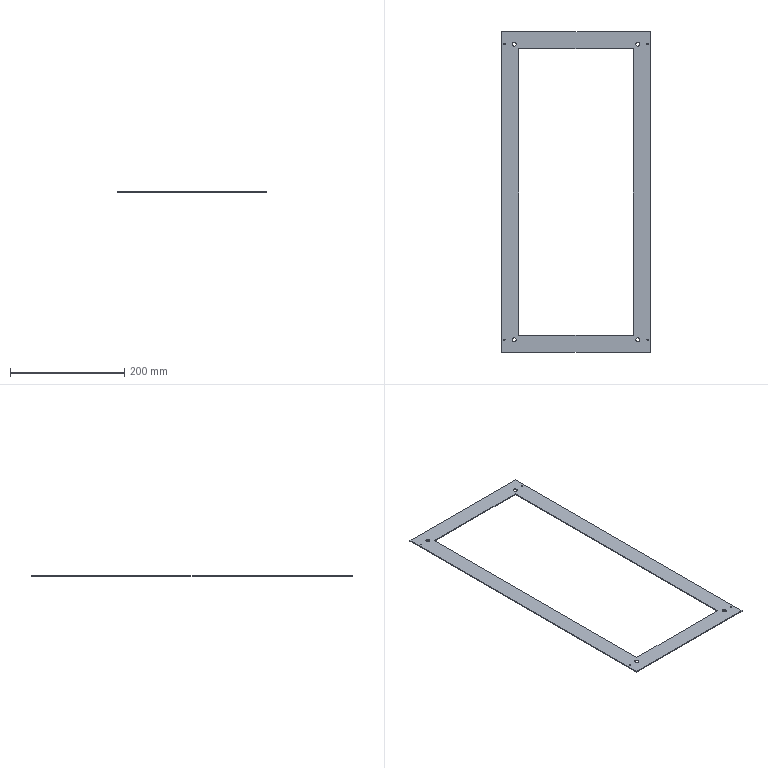Part | SolidWorks | features Cut 2, FlatPattern 1, LPattern 1, SMBaseFlange 1, SheetMetal 1 | 1 solid | 26 faces | box 260 x 560.2 x 1.5 mm | volume 68162 mm3 | cylinder 16 | plane 10 | commonest cylinder face diameters 2 x8 7.1 x8
STEP:
#1=CARTESIAN_POINT('',(234.45,538.2,-1.5));
#2=VERTEX_POINT('',#1);
#3=CARTESIAN_POINT('',(241.55,538.2,-1.5));
#4=VERTEX_POINT('',#3);
#5=CARTESIAN_POINT('',(238.,538.2,-1.5));
#6=DIRECTION('',(0.,0.,1.));
#7=DIRECTION('',(1.,0.,0.));
#8=AXIS2_PLACEMENT_3D('',#5,#6,#7);
#9=CIRCLE('',#8,3.55);
#10=EDGE_CURVE('',#2,#4,#9,.T.);
#11=ORIENTED_EDGE('',*,*,#10,.F.);
#12=CARTESIAN_POINT('',(234.45,538.2,0.));
#13=VERTEX_POINT('',#12);
#14=CARTESIAN_POINT('',(234.45,538.2,-1.5));
#15=DIRECTION('',(0.,0.,1.));
#16=VECTOR('',#15,1000.);
#17=LINE('',#14,#16);
#18=EDGE_CURVE('',#2,#13,#17,.T.);
#19=ORIENTED_EDGE('',*,*,#18,.T.);
#20=CARTESIAN_POINT('',(241.55,538.2,0.));
#21=VERTEX_POINT('',#20);
#22=CARTESIAN_POINT('',(238.,538.2,0.));
#23=DIRECTION('',(0.,0.,1.));
#24=DIRECTION('',(1.,0.,0.));
#25=AXIS2_PLACEMENT_3D('',#22,#23,#24);
#26=CIRCLE('',#25,3.55);
#27=EDGE_CURVE('',#13,#21,#26,.T.);
#28=ORIENTED_EDGE('',*,*,#27,.T.);
#29=CARTESIAN_POINT('',(241.55,538.2,-1.5));
#30=DIRECTION('',(0.,0.,1.));
#31=VECTOR('',#30,1000.);
#32=LINE('',#29,#31);
#33=EDGE_CURVE('',#4,#21,#32,.T.);
#34=ORIENTED_EDGE('',*,*,#33,.F.);
#35=EDGE_LOOP('',(#11,#19,#28,#34));
#36=FACE_OUTER_BOUND('',#35,.T.);
#37=CARTESIAN_POINT('',(238.,538.2,-1.5));
#38=DIRECTION('',(0.,0.,1.));
#39=DIRECTION('',(1.,0.,0.));
#40=AXIS2_PLACEMENT_3D('',#37,#38,#39);
#41=CYLINDRICAL_SURFACE('',#40,3.55);
#42=ADVANCED_FACE('',(#36),#41,.F.);
#43=CARTESIAN_POINT('',(18.45,538.2,-1.5));
#44=VERTEX_POINT('',#43);
#45=CARTESIAN_POINT('',(25.55,538.2,-1.5));
#46=VERTEX_POINT('',#45);
#47=CARTESIAN_POINT('',(22.,538.2,-1.5));
#48=DIRECTION('',(0.,0.,1.));
#49=DIRECTION('',(1.,0.,0.));
#50=AXIS2_PLACEMENT_3D('',#47,#48,#49);
#51=CIRCLE('',#50,3.55);
#52=EDGE_CURVE('',#44,#46,#51,.T.);
#53=ORIENTED_EDGE('',*,*,#52,.F.);
#54=CARTESIAN_POINT('',(18.45,538.2,0.));
#55=VERTEX_POINT('',#54);
#56=CARTESIAN_POINT('',(18.45,538.2,-1.5));
#57=DIRECTION('',(0.,0.,1.));
#58=VECTOR('',#57,1000.);
#59=LINE('',#56,#58);
#60=EDGE_CURVE('',#44,#55,#59,.T.);
#61=ORIENTED_EDGE('',*,*,#60,.T.);
#62=CARTESIAN_POINT('',(25.55,538.2,0.));
#63=VERTEX_POINT('',#62);
#64=CARTESIAN_POINT('',(22.,538.2,0.));
#65=DIRECTION('',(0.,0.,1.));
#66=DIRECTION('',(1.,0.,0.));
#67=AXIS2_PLACEMENT_3D('',#64,#65,#66);
#68=CIRCLE('',#67,3.55);
#69=EDGE_CURVE('',#55,#63,#68,.T.);
#70=ORIENTED_EDGE('',*,*,#69,.T.);
#71=CARTESIAN_POINT('',(25.55,538.2,-1.5));
#72=DIRECTION('',(0.,0.,1.));
#73=VECTOR('',#72,1000.);
#74=LINE('',#71,#73);
#75=EDGE_CURVE('',#46,#63,#74,.T.);
#76=ORIENTED_EDGE('',*,*,#75,.F.);
#77=EDGE_LOOP('',(#53,#61,#70,#76));
#78=FACE_OUTER_BOUND('',#77,.T.);
#79=CARTESIAN_POINT('',(22.,538.2,-1.5));
#80=DIRECTION('',(0.,0.,1.));
#81=DIRECTION('',(1.,0.,0.));
#82=AXIS2_PLACEMENT_3D('',#79,#80,#81);
#83=CYLINDRICAL_SURFACE('',#82,3.55);
#84=ADVANCED_FACE('',(#78),#83,.F.);
#85=CARTESIAN_POINT('',(18.45,22.,-1.5));
#86=VERTEX_POINT('',#85);
#87=CARTESIAN_POINT('',(25.55,22.,-1.5));
#88=VERTEX_POINT('',#87);
#89=CARTESIAN_POINT('',(22.,22.,-1.5));
#90=DIRECTION('',(0.,0.,1.));
#91=DIRECTION('',(1.,0.,0.));
#92=AXIS2_PLACEMENT_3D('',#89,#90,#91);
#93=CIRCLE('',#92,3.55);
#94=EDGE_CURVE('',#86,#88,#93,.T.);
#95=ORIENTED_EDGE('',*,*,#94,.F.);
#96=CARTESIAN_POINT('',(18.45,22.,0.));
#97=VERTEX_POINT('',#96);
#98=CARTESIAN_POINT('',(18.45,22.,-1.5));
#99=DIRECTION('',(0.,0.,1.));
#100=VECTOR('',#99,1000.);
#101=LINE('',#98,#100);
#102=EDGE_CURVE('',#86,#97,#101,.T.);
#103=ORIENTED_EDGE('',*,*,#102,.T.);
#104=CARTESIAN_POINT('',(25.55,22.,0.));
#105=VERTEX_POINT('',#104);
#106=CARTESIAN_POINT('',(22.,22.,0.));
#107=DIRECTION('',(0.,0.,1.));
#108=DIRECTION('',(1.,0.,0.));
#109=AXIS2_PLACEMENT_3D('',#106,#107,#108);
#110=CIRCLE('',#109,3.55);
#111=EDGE_CURVE('',#97,#105,#110,.T.);
#112=ORIENTED_EDGE('',*,*,#111,.T.);
#113=CARTESIAN_POINT('',(25.55,22.,-1.5));
#114=DIRECTION('',(0.,0.,1.));
#115=VECTOR('',#114,1000.);
#116=LINE('',#113,#115);
#117=EDGE_CURVE('',#88,#105,#116,.T.);
#118=ORIENTED_EDGE('',*,*,#117,.F.);
#119=EDGE_LOOP('',(#95,#103,#112,#118));
#120=FACE_OUTER_BOUND('',#119,.T.);
#121=CARTESIAN_POINT('',(22.,22.,-1.5));
#122=DIRECTION('',(0.,0.,1.));
#123=DIRECTION('',(1.,0.,0.));
#124=AXIS2_PLACEMENT_3D('',#121,#122,#123);
#125=CYLINDRICAL_SURFACE('',#124,3.55);
#126=ADVANCED_FACE('',(#120),#125,.F.);
#127=CARTESIAN_POINT('',(234.45,22.,-1.5));
#128=VERTEX_POINT('',#127);
#129=CARTESIAN_POINT('',(241.55,22.,-1.5));
#130=VERTEX_POINT('',#129);
#131=CARTESIAN_POINT('',(238.,22.,-1.5));
#132=DIRECTION('',(0.,0.,1.));
#133=DIRECTION('',(1.,0.,0.));
#134=AXIS2_PLACEMENT_3D('',#131,#132,#133);
#135=CIRCLE('',#134,3.55);
#136=EDGE_CURVE('',#128,#130,#135,.T.);
#137=ORIENTED_EDGE('',*,*,#136,.F.);
#138=CARTESIAN_POINT('',(234.45,22.,0.));
#139=VERTEX_POINT('',#138);
#140=CARTESIAN_POINT('',(234.45,22.,-1.5));
#141=DIRECTION('',(0.,0.,1.));
#142=VECTOR('',#141,1000.);
#143=LINE('',#140,#142);
#144=EDGE_CURVE('',#128,#139,#143,.T.);
#145=ORIENTED_EDGE('',*,*,#144,.T.);
#146=CARTESIAN_POINT('',(241.55,22.,0.));
#147=VERTEX_POINT('',#146);
#148=CARTESIAN_POINT('',(238.,22.,0.));
#149=DIRECTION('',(0.,0.,1.));
#150=DIRECTION('',(1.,0.,0.));
#151=AXIS2_PLACEMENT_3D('',#148,#149,#150);
#152=CIRCLE('',#151,3.55);
#153=EDGE_CURVE('',#139,#147,#152,.T.);
#154=ORIENTED_EDGE('',*,*,#153,.T.);
#155=CARTESIAN_POINT('',(241.55,22.,-1.5));
#156=DIRECTION('',(0.,0.,1.));
#157=VECTOR('',#156,1000.);
#158=LINE('',#155,#157);
#159=EDGE_CURVE('',#130,#147,#158,.T.);
#160=ORIENTED_EDGE('',*,*,#159,.F.);
#161=EDGE_LOOP('',(#137,#145,#154,#160));
#162=FACE_OUTER_BOUND('',#161,.T.);
#163=CARTESIAN_POINT('',(238.,22.,-1.5));
#164=DIRECTION('',(0.,0.,1.));
#165=DIRECTION('',(1.,0.,0.));
#166=AXIS2_PLACEMENT_3D('',#163,#164,#165);
#167=CYLINDRICAL_SURFACE('',#166,3.55);
#168=ADVANCED_FACE('',(#162),#167,.F.);
#169=CARTESIAN_POINT('',(4.,22.,-1.5));
#170=VERTEX_POINT('',#169);
#171=CARTESIAN_POINT('',(6.,22.,-1.5));
#172=VERTEX_POINT('',#171);
#173=CARTESIAN_POINT('',(5.,22.,-1.5));
#174=DIRECTION('',(0.,0.,1.));
#175=DIRECTION('',(1.,0.,0.));
#176=AXIS2_PLACEMENT_3D('',#173,#174,#175);
#177=CIRCLE('',#176,1.);
#178=EDGE_CURVE('',#170,#172,#177,.T.);
#179=ORIENTED_EDGE('',*,*,#178,.F.);
#180=CARTESIAN_POINT('',(4.,22.,0.));
#181=VERTEX_POINT('',#180);
#182=CARTESIAN_POINT('',(4.,22.,-1.5));
#183=DIRECTION('',(0.,0.,1.));
#184=VECTOR('',#183,1000.);
#185=LINE('',#182,#184);
#186=EDGE_CURVE('',#170,#181,#185,.T.);
#187=ORIENTED_EDGE('',*,*,#186,.T.);
#188=CARTESIAN_POINT('',(6.,22.,0.));
#189=VERTEX_POINT('',#188);
#190=CARTESIAN_POINT('',(5.,22.,0.));
#191=DIRECTION('',(0.,0.,1.));
#192=DIRECTION('',(1.,0.,0.));
#193=AXIS2_PLACEMENT_3D('',#190,#191,#192);
#194=CIRCLE('',#193,1.);
#195=EDGE_CURVE('',#181,#189,#194,.T.);
#196=ORIENTED_EDGE('',*,*,#195,.T.);
#197=CARTESIAN_POINT('',(6.,22.,-1.5));
#198=DIRECTION('',(0.,0.,1.));
#199=VECTOR('',#198,1000.);
#200=LINE('',#197,#199);
#201=EDGE_CURVE('',#172,#189,#200,.T.);
#202=ORIENTED_EDGE('',*,*,#201,.F.);
#203=EDGE_LOOP('',(#179,#187,#196,#202));
#204=FACE_OUTER_BOUND('',#203,.T.);
#205=CARTESIAN_POINT('',(5.,22.,-1.5));
#206=DIRECTION('',(0.,0.,1.));
#207=DIRECTION('',(1.,0.,0.));
#208=AXIS2_PLACEMENT_3D('',#205,#206,#207);
#209=CYLINDRICAL_SURFACE('',#208,1.);
#210=ADVANCED_FACE('',(#204),#209,.F.);
#211=CARTESIAN_POINT('',(254.,22.,-1.5));
#212=VERTEX_POINT('',#211);
#213=CARTESIAN_POINT('',(256.,22.,-1.5));
#214=VERTEX_POINT('',#213);
#215=CARTESIAN_POINT('',(255.,22.,-1.5));
#216=DIRECTION('',(0.,0.,1.));
#217=DIRECTION('',(1.,0.,0.));
#218=AXIS2_PLACEMENT_3D('',#215,#216,#217);
#219=CIRCLE('',#218,1.);
#220=EDGE_CURVE('',#212,#214,#219,.T.);
#221=ORIENTED_EDGE('',*,*,#220,.F.);
#222=CARTESIAN_POINT('',(254.,22.,0.));
#223=VERTEX_POINT('',#222);
#224=CARTESIAN_POINT('',(254.,22.,-1.5));
#225=DIRECTION('',(0.,0.,1.));
#226=VECTOR('',#225,1000.);
#227=LINE('',#224,#226);
#228=EDGE_CURVE('',#212,#223,#227,.T.);
#229=ORIENTED_EDGE('',*,*,#228,.T.);
#230=CARTESIAN_POINT('',(256.,22.,0.));
#231=VERTEX_POINT('',#230);
#232=CARTESIAN_POINT('',(255.,22.,0.));
#233=DIRECTION('',(0.,0.,1.));
#234=DIRECTION('',(1.,0.,0.));
#235=AXIS2_PLACEMENT_3D('',#232,#233,#234);
#236=CIRCLE('',#235,1.);
#237=EDGE_CURVE('',#223,#231,#236,.T.);
#238=ORIENTED_EDGE('',*,*,#237,.T.);
#239=CARTESIAN_POINT('',(256.,22.,-1.5));
#240=DIRECTION('',(0.,0.,1.));
#241=VECTOR('',#240,1000.);
#242=LINE('',#239,#241);
#243=EDGE_CURVE('',#214,#231,#242,.T.);
#244=ORIENTED_EDGE('',*,*,#243,.F.);
#245=EDGE_LOOP('',(#221,#229,#238,#244));
#246=FACE_OUTER_BOUND('',#245,.T.);
#247=CARTESIAN_POINT('',(255.,22.,-1.5));
#248=DIRECTION('',(0.,0.,1.));
#249=DIRECTION('',(1.,0.,0.));
#250=AXIS2_PLACEMENT_3D('',#247,#248,#249);
#251=CYLINDRICAL_SURFACE('',#250,1.);
#252=ADVANCED_FACE('',(#246),#251,.F.);
#253=CARTESIAN_POINT('',(254.,538.6,-1.5));
#254=VERTEX_POINT('',#253);
#255=CARTESIAN_POINT('',(256.,538.6,-1.5));
#256=VERTEX_POINT('',#255);
#257=CARTESIAN_POINT('',(255.,538.6,-1.5));
#258=DIRECTION('',(0.,0.,1.));
#259=DIRECTION('',(1.,0.,0.));
#260=AXIS2_PLACEMENT_3D('',#257,#258,#259);
#261=CIRCLE('',#260,1.);
#262=EDGE_CURVE('',#254,#256,#261,.T.);
#263=ORIENTED_EDGE('',*,*,#262,.F.);
#264=CARTESIAN_POINT('',(254.,538.6,0.));
#265=VERTEX_POINT('',#264);
#266=CARTESIAN_POINT('',(254.,538.6,-1.5));
#267=DIRECTION('',(0.,0.,1.));
#268=VECTOR('',#267,1000.);
#269=LINE('',#266,#268);
#270=EDGE_CURVE('',#254,#265,#269,.T.);
#271=ORIENTED_EDGE('',*,*,#270,.T.);
#272=CARTESIAN_POINT('',(256.,538.6,0.));
#273=VERTEX_POINT('',#272);
#274=CARTESIAN_POINT('',(255.,538.6,0.));
#275=DIRECTION('',(0.,0.,1.));
#276=DIRECTION('',(1.,0.,0.));
#277=AXIS2_PLACEMENT_3D('',#274,#275,#276);
#278=CIRCLE('',#277,1.);
#279=EDGE_CURVE('',#265,#273,#278,.T.);
#280=ORIENTED_EDGE('',*,*,#279,.T.);
#281=CARTESIAN_POINT('',(256.,538.6,-1.5));
#282=DIRECTION('',(0.,0.,1.));
#283=VECTOR('',#282,1000.);
#284=LINE('',#281,#283);
#285=EDGE_CURVE('',#256,#273,#284,.T.);
#286=ORIENTED_EDGE('',*,*,#285,.F.);
#287=EDGE_LOOP('',(#263,#271,#280,#286));
#288=FACE_OUTER_BOUND('',#287,.T.);
#289=CARTESIAN_POINT('',(255.,538.6,-1.5));
#290=DIRECTION('',(0.,0.,1.));
#291=DIRECTION('',(1.,0.,0.));
#292=AXIS2_PLACEMENT_3D('',#289,#290,#291);
#293=CYLINDRICAL_SURFACE('',#292,1.);
#294=ADVANCED_FACE('',(#288),#293,.F.);
#295=CARTESIAN_POINT('',(4.,538.6,-1.5));
#296=VERTEX_POINT('',#295);
#297=CARTESIAN_POINT('',(6.,538.6,-1.5));
#298=VERTEX_POINT('',#297);
#299=CARTESIAN_POINT('',(5.,538.6,-1.5));
#300=DIRECTION('',(0.,0.,1.));
#301=DIRECTION('',(1.,0.,0.));
#302=AXIS2_PLACEMENT_3D('',#299,#300,#301);
#303=CIRCLE('',#302,1.);
#304=EDGE_CURVE('',#296,#298,#303,.T.);
#305=ORIENTED_EDGE('',*,*,#304,.F.);
#306=CARTESIAN_POINT('',(4.,538.6,0.));
#307=VERTEX_POINT('',#306);
#308=CARTESIAN_POINT('',(4.,538.6,-1.5));
#309=DIRECTION('',(0.,0.,1.));
#310=VECTOR('',#309,1000.);
#311=LINE('',#308,#310);
#312=EDGE_CURVE('',#296,#307,#311,.T.);
#313=ORIENTED_EDGE('',*,*,#312,.T.);
#314=CARTESIAN_POINT('',(6.,538.6,0.));
#315=VERTEX_POINT('',#314);
#316=CARTESIAN_POINT('',(5.,538.6,0.));
#317=DIRECTION('',(0.,0.,1.));
#318=DIRECTION('',(1.,0.,0.));
#319=AXIS2_PLACEMENT_3D('',#316,#317,#318);
#320=CIRCLE('',#319,1.);
#321=EDGE_CURVE('',#307,#315,#320,.T.);
#322=ORIENTED_EDGE('',*,*,#321,.T.);
#323=CARTESIAN_POINT('',(6.,538.6,-1.5));
#324=DIRECTION('',(0.,0.,1.));
#325=VECTOR('',#324,1000.);
#326=LINE('',#323,#325);
#327=EDGE_CURVE('',#298,#315,#326,.T.);
#328=ORIENTED_EDGE('',*,*,#327,.F.);
#329=EDGE_LOOP('',(#305,#313,#322,#328));
#330=FACE_OUTER_BOUND('',#329,.T.);
#331=CARTESIAN_POINT('',(5.,538.6,-1.5));
#332=DIRECTION('',(0.,0.,1.));
#333=DIRECTION('',(1.,0.,0.));
#334=AXIS2_PLACEMENT_3D('',#331,#332,#333);
#335=CYLINDRICAL_SURFACE('',#334,1.);
#336=ADVANCED_FACE('',(#330),#335,.F.);
#337=ORIENTED_EDGE('',*,*,#312,.F.);
#338=CARTESIAN_POINT('',(5.,538.6,-1.5));
#339=DIRECTION('',(0.,0.,1.));
#340=DIRECTION('',(1.,0.,0.));
#341=AXIS2_PLACEMENT_3D('',#338,#339,#340);
#342=CIRCLE('',#341,1.);
#343=EDGE_CURVE('',#298,#296,#342,.T.);
#344=ORIENTED_EDGE('',*,*,#343,.F.);
#345=ORIENTED_EDGE('',*,*,#327,.T.);
#346=CARTESIAN_POINT('',(5.,538.6,0.));
#347=DIRECTION('',(0.,0.,1.));
#348=DIRECTION('',(1.,0.,0.));
#349=AXIS2_PLACEMENT_3D('',#346,#347,#348);
#350=CIRCLE('',#349,1.);
#351=EDGE_CURVE('',#315,#307,#350,.T.);
#352=ORIENTED_EDGE('',*,*,#351,.T.);
#353=EDGE_LOOP('',(#337,#344,#345,#352));
#354=FACE_OUTER_BOUND('',#353,.T.);
#355=CARTESIAN_POINT('',(5.,538.6,-1.5));
#356=DIRECTION('',(0.,0.,1.));
#357=DIRECTION('',(1.,0.,0.));
#358=AXIS2_PLACEMENT_3D('',#355,#356,#357);
#359=CYLINDRICAL_SURFACE('',#358,1.);
#360=ADVANCED_FACE('',(#354),#359,.F.);
#361=ORIENTED_EDGE('',*,*,#270,.F.);
#362=CARTESIAN_POINT('',(255.,538.6,-1.5));
#363=DIRECTION('',(0.,0.,1.));
#364=DIRECTION('',(1.,0.,0.));
#365=AXIS2_PLACEMENT_3D('',#362,#363,#364);
#366=CIRCLE('',#365,1.);
#367=EDGE_CURVE('',#256,#254,#366,.T.);
#368=ORIENTED_EDGE('',*,*,#367,.F.);
#369=ORIENTED_EDGE('',*,*,#285,.T.);
#370=CARTESIAN_POINT('',(255.,538.6,0.));
#371=DIRECTION('',(0.,0.,1.));
#372=DIRECTION('',(1.,0.,0.));
#373=AXIS2_PLACEMENT_3D('',#370,#371,#372);
#374=CIRCLE('',#373,1.);
#375=EDGE_CURVE('',#273,#265,#374,.T.);
#376=ORIENTED_EDGE('',*,*,#375,.T.);
#377=EDGE_LOOP('',(#361,#368,#369,#376));
#378=FACE_OUTER_BOUND('',#377,.T.);
#379=CARTESIAN_POINT('',(255.,538.6,-1.5));
#380=DIRECTION('',(0.,0.,1.));
#381=DIRECTION('',(1.,0.,0.));
#382=AXIS2_PLACEMENT_3D('',#379,#380,#381);
#383=CYLINDRICAL_SURFACE('',#382,1.);
#384=ADVANCED_FACE('',(#378),#383,.F.);
#385=CARTESIAN_POINT('',(0.,560.2,0.));
#386=VERTEX_POINT('',#385);
#387=CARTESIAN_POINT('',(0.,0.,0.));
#388=VERTEX_POINT('',#387);
#389=CARTESIAN_POINT('',(0.,0.,0.));
#390=DIRECTION('',(0.,-1.,0.));
#391=VECTOR('',#390,1000.);
#392=LINE('',#389,#391);
#393=EDGE_CURVE('',#386,#388,#392,.T.);
#394=ORIENTED_EDGE('',*,*,#393,.F.);
#395=CARTESIAN_POINT('',(0.,560.2,-1.5));
#396=VERTEX_POINT('',#395);
#397=CARTESIAN_POINT('',(0.,560.2,-1.5));
#398=DIRECTION('',(0.,0.,1.));
#399=VECTOR('',#398,1000.);
#400=LINE('',#397,#399);
#401=EDGE_CURVE('',#396,#386,#400,.T.);
#402=ORIENTED_EDGE('',*,*,#401,.F.);
#403=CARTESIAN_POINT('',(0.,0.,-1.5));
#404=VERTEX_POINT('',#403);
#405=CARTESIAN_POINT('',(0.,0.,-1.5));
#406=DIRECTION('',(0.,-1.,0.));
#407=VECTOR('',#406,1000.);
#408=LINE('',#405,#407);
#409=EDGE_CURVE('',#396,#404,#408,.T.);
#410=ORIENTED_EDGE('',*,*,#409,.T.);
#411=CARTESIAN_POINT('',(0.,0.,-1.5));
#412=DIRECTION('',(0.,0.,1.));
#413=VECTOR('',#412,1000.);
#414=LINE('',#411,#413);
#415=EDGE_CURVE('',#404,#388,#414,.T.);
#416=ORIENTED_EDGE('',*,*,#415,.T.);
#417=EDGE_LOOP('',(#394,#402,#410,#416));
#418=FACE_OUTER_BOUND('',#417,.T.);
#419=CARTESIAN_POINT('',(0.,0.,-1.5));
#420=DIRECTION('',(-1.,0.,0.));
#421=DIRECTION('',(0.,-1.,0.));
#422=AXIS2_PLACEMENT_3D('',#419,#420,#421);
#423=PLANE('',#422);
#424=ADVANCED_FACE('',(#418),#423,.T.);
#425=CARTESIAN_POINT('',(260.,560.2,0.));
#426=VERTEX_POINT('',#425);
#427=CARTESIAN_POINT('',(0.,560.2,0.));
#428=DIRECTION('',(-1.,0.,0.));
#429=VECTOR('',#428,1000.);
#430=LINE('',#427,#429);
#431=EDGE_CURVE('',#426,#386,#430,.T.);
#432=ORIENTED_EDGE('',*,*,#431,.F.);
#433=CARTESIAN_POINT('',(260.,560.2,-1.5));
#434=VERTEX_POINT('',#433);
#435=CARTESIAN_POINT('',(260.,560.2,-1.5));
#436=DIRECTION('',(0.,0.,1.));
#437=VECTOR('',#436,1000.);
#438=LINE('',#435,#437);
#439=EDGE_CURVE('',#434,#426,#438,.T.);
#440=ORIENTED_EDGE('',*,*,#439,.F.);
#441=CARTESIAN_POINT('',(0.,560.2,-1.5));
#442=DIRECTION('',(-1.,0.,0.));
#443=VECTOR('',#442,1000.);
#444=LINE('',#441,#443);
#445=EDGE_CURVE('',#434,#396,#444,.T.);
#446=ORIENTED_EDGE('',*,*,#445,.T.);
#447=ORIENTED_EDGE('',*,*,#401,.T.);
#448=EDGE_LOOP('',(#432,#440,#446,#447));
#449=FACE_OUTER_BOUND('',#448,.T.);
#450=CARTESIAN_POINT('',(0.,560.2,-1.5));
#451=DIRECTION('',(0.,1.,0.));
#452=DIRECTION('',(0.,0.,1.));
#453=AXIS2_PLACEMENT_3D('',#450,#451,#452);
#454=PLANE('',#453);
#455=ADVANCED_FACE('',(#449),#454,.T.);
#456=CARTESIAN_POINT('',(260.,0.,0.));
#457=VERTEX_POINT('',#456);
#458=CARTESIAN_POINT('',(260.,0.,0.));
#459=DIRECTION('',(0.,1.,0.));
#460=VECTOR('',#459,1000.);
#461=LINE('',#458,#460);
#462=EDGE_CURVE('',#457,#426,#461,.T.);
#463=ORIENTED_EDGE('',*,*,#462,.F.);
#464=CARTESIAN_POINT('',(260.,0.,-1.5));
#465=VERTEX_POINT('',#464);
#466=CARTESIAN_POINT('',(260.,0.,-1.5));
#467=DIRECTION('',(0.,0.,1.));
#468=VECTOR('',#467,1000.);
#469=LINE('',#466,#468);
#470=EDGE_CURVE('',#465,#457,#469,.T.);
#471=ORIENTED_EDGE('',*,*,#470,.F.);
#472=CARTESIAN_POINT('',(260.,0.,-1.5));
#473=DIRECTION('',(0.,1.,0.));
#474=VECTOR('',#473,1000.);
#475=LINE('',#472,#474);
#476=EDGE_CURVE('',#465,#434,#475,.T.);
#477=ORIENTED_EDGE('',*,*,#476,.T.);
#478=ORIENTED_EDGE('',*,*,#439,.T.);
#479=EDGE_LOOP('',(#463,#471,#477,#478));
#480=FACE_OUTER_BOUND('',#479,.T.);
#481=CARTESIAN_POINT('',(260.,0.,-1.5));
#482=DIRECTION('',(1.,0.,0.));
#483=DIRECTION('',(0.,1.,0.));
#484=AXIS2_PLACEMENT_3D('',#481,#482,#483);
#485=PLANE('',#484);
#486=ADVANCED_FACE('',(#480),#485,.T.);
#487=CARTESIAN_POINT('',(0.,0.,0.));
#488=DIRECTION('',(1.,0.,0.));
#489=VECTOR('',#488,1000.);
#490=LINE('',#487,#489);
#491=EDGE_CURVE('',#388,#457,#490,.T.);
#492=ORIENTED_EDGE('',*,*,#491,.F.);
#493=ORIENTED_EDGE('',*,*,#415,.F.);
#494=CARTESIAN_POINT('',(0.,0.,-1.5));
#495=DIRECTION('',(1.,0.,0.));
#496=VECTOR('',#495,1000.);
#497=LINE('',#494,#496);
#498=EDGE_CURVE('',#404,#465,#497,.T.);
#499=ORIENTED_EDGE('',*,*,#498,.T.);
#500=ORIENTED_EDGE('',*,*,#470,.T.);
#501=EDGE_LOOP('',(#492,#493,#499,#500));
#502=FACE_OUTER_BOUND('',#501,.T.);
#503=CARTESIAN_POINT('',(0.,0.,-1.5));
#504=DIRECTION('',(0.,-1.,0.));
#505=DIRECTION('',(0.,0.,-1.));
#506=AXIS2_PLACEMENT_3D('',#503,#504,#505);
#507=PLANE('',#506);
#508=ADVANCED_FACE('',(#502),#507,.T.);
#509=CARTESIAN_POINT('',(238.,538.2,-1.5));
#510=DIRECTION('',(0.,0.,1.));
#511=DIRECTION('',(1.,0.,0.));
#512=AXIS2_PLACEMENT_3D('',#509,#510,#511);
#513=CIRCLE('',#512,3.55);
#514=EDGE_CURVE('',#4,#2,#513,.T.);
#515=ORIENTED_EDGE('',*,*,#514,.T.);
#516=ORIENTED_EDGE('',*,*,#10,.T.);
#517=EDGE_LOOP('',(#515,#516));
#518=FACE_BOUND('',#517,.T.);
#519=CARTESIAN_POINT('',(22.,538.2,-1.5));
#520=DIRECTION('',(0.,0.,1.));
#521=DIRECTION('',(1.,0.,0.));
#522=AXIS2_PLACEMENT_3D('',#519,#520,#521);
#523=CIRCLE('',#522,3.55);
#524=EDGE_CURVE('',#46,#44,#523,.T.);
#525=ORIENTED_EDGE('',*,*,#524,.T.);
#526=ORIENTED_EDGE('',*,*,#52,.T.);
#527=EDGE_LOOP('',(#525,#526));
#528=FACE_BOUND('',#527,.T.);
#529=CARTESIAN_POINT('',(22.,22.,-1.5));
#530=DIRECTION('',(0.,0.,1.));
#531=DIRECTION('',(1.,0.,0.));
#532=AXIS2_PLACEMENT_3D('',#529,#530,#531);
#533=CIRCLE('',#532,3.55);
#534=EDGE_CURVE('',#88,#86,#533,.T.);
#535=ORIENTED_EDGE('',*,*,#534,.T.);
#536=ORIENTED_EDGE('',*,*,#94,.T.);
#537=EDGE_LOOP('',(#535,#536));
#538=FACE_BOUND('',#537,.T.);
#539=CARTESIAN_POINT('',(238.,22.,-1.5));
#540=DIRECTION('',(0.,0.,1.));
#541=DIRECTION('',(1.,0.,0.));
#542=AXIS2_PLACEMENT_3D('',#539,#540,#541);
#543=CIRCLE('',#542,3.55);
#544=EDGE_CURVE('',#130,#128,#543,.T.);
#545=ORIENTED_EDGE('',*,*,#544,.T.);
#546=ORIENTED_EDGE('',*,*,#136,.T.);
#547=EDGE_LOOP('',(#545,#546));
#548=FACE_BOUND('',#547,.T.);
#549=CARTESIAN_POINT('',(5.,22.,-1.5));
#550=DIRECTION('',(0.,0.,1.));
#551=DIRECTION('',(1.,0.,0.));
#552=AXIS2_PLACEMENT_3D('',#549,#550,#551);
#553=CIRCLE('',#552,1.);
#554=EDGE_CURVE('',#172,#170,#553,.T.);
#555=ORIENTED_EDGE('',*,*,#554,.T.);
#556=ORIENTED_EDGE('',*,*,#178,.T.);
#557=EDGE_LOOP('',(#555,#556));
#558=FACE_BOUND('',#557,.T.);
#559=CARTESIAN_POINT('',(255.,22.,-1.5));
#560=DIRECTION('',(0.,0.,1.));
#561=DIRECTION('',(1.,0.,0.));
#562=AXIS2_PLACEMENT_3D('',#559,#560,#561);
#563=CIRCLE('',#562,1.);
#564=EDGE_CURVE('',#214,#212,#563,.T.);
#565=ORIENTED_EDGE('',*,*,#564,.T.);
#566=ORIENTED_EDGE('',*,*,#220,.T.);
#567=EDGE_LOOP('',(#565,#566));
#568=FACE_BOUND('',#567,.T.);
#569=CARTESIAN_POINT('',(30.,530.2,-1.5));
#570=VERTEX_POINT('',#569);
#571=CARTESIAN_POINT('',(30.,30.,-1.5));
#572=VERTEX_POINT('',#571);
#573=CARTESIAN_POINT('',(30.,30.,-1.5));
#574=DIRECTION('',(0.,-1.,0.));
#575=VECTOR('',#574,1000.);
#576=LINE('',#573,#575);
#577=EDGE_CURVE('',#570,#572,#576,.T.);
#578=ORIENTED_EDGE('',*,*,#577,.T.);
#579=CARTESIAN_POINT('',(230.,30.,-1.5));
#580=VERTEX_POINT('',#579);
#581=CARTESIAN_POINT('',(30.,30.,-1.5));
#582=DIRECTION('',(1.,0.,0.));
#583=VECTOR('',#582,1000.);
#584=LINE('',#581,#583);
#585=EDGE_CURVE('',#572,#580,#584,.T.);
#586=ORIENTED_EDGE('',*,*,#585,.T.);
#587=CARTESIAN_POINT('',(230.,530.2,-1.5));
#588=VERTEX_POINT('',#587);
#589=CARTESIAN_POINT('',(230.,30.,-1.5));
#590=DIRECTION('',(0.,1.,0.));
#591=VECTOR('',#590,1000.);
#592=LINE('',#589,#591);
#593=EDGE_CURVE('',#580,#588,#592,.T.);
#594=ORIENTED_EDGE('',*,*,#593,.T.);
#595=CARTESIAN_POINT('',(30.,530.2,-1.5));
#596=DIRECTION('',(-1.,0.,0.));
#597=VECTOR('',#596,1000.);
#598=LINE('',#595,#597);
#599=EDGE_CURVE('',#588,#570,#598,.T.);
#600=ORIENTED_EDGE('',*,*,#599,.T.);
#601=EDGE_LOOP('',(#578,#586,#594,#600));
#602=FACE_BOUND('',#601,.T.);
#603=ORIENTED_EDGE('',*,*,#409,.F.);
#604=ORIENTED_EDGE('',*,*,#445,.F.);
#605=ORIENTED_EDGE('',*,*,#476,.F.);
#606=ORIENTED_EDGE('',*,*,#498,.F.);
#607=EDGE_LOOP('',(#603,#604,#605,#606));
#608=FACE_OUTER_BOUND('',#607,.T.);
#609=ORIENTED_EDGE('',*,*,#367,.T.);
#610=ORIENTED_EDGE('',*,*,#262,.T.);
#611=EDGE_LOOP('',(#609,#610));
#612=FACE_BOUND('',#611,.T.);
#613=ORIENTED_EDGE('',*,*,#343,.T.);
#614=ORIENTED_EDGE('',*,*,#304,.T.);
#615=EDGE_LOOP('',(#613,#614));
#616=FACE_BOUND('',#615,.T.);
#617=CARTESIAN_POINT('',(0.,0.,-1.5));
#618=DIRECTION('',(0.,0.,-1.));
#619=DIRECTION('',(-1.,0.,0.));
#620=AXIS2_PLACEMENT_3D('',#617,#618,#619);
#621=PLANE('',#620);
#622=ADVANCED_FACE('',(#518,#528,#538,#548,#558,#568,#602,#608,#612,#616),#621,.T.);
#623=CARTESIAN_POINT('',(238.,538.2,0.));
#624=DIRECTION('',(0.,0.,1.));
#625=DIRECTION('',(1.,0.,0.));
#626=AXIS2_PLACEMENT_3D('',#623,#624,#625);
#627=CIRCLE('',#626,3.55);
#628=EDGE_CURVE('',#21,#13,#627,.T.);
#629=ORIENTED_EDGE('',*,*,#628,.F.);
#630=ORIENTED_EDGE('',*,*,#27,.F.);
#631=EDGE_LOOP('',(#629,#630));
#632=FACE_BOUND('',#631,.T.);
#633=CARTESIAN_POINT('',(22.,538.2,0.));
#634=DIRECTION('',(0.,0.,1.));
#635=DIRECTION('',(1.,0.,0.));
#636=AXIS2_PLACEMENT_3D('',#633,#634,#635);
#637=CIRCLE('',#636,3.55);
#638=EDGE_CURVE('',#63,#55,#637,.T.);
#639=ORIENTED_EDGE('',*,*,#638,.F.);
#640=ORIENTED_EDGE('',*,*,#69,.F.);
#641=EDGE_LOOP('',(#639,#640));
#642=FACE_BOUND('',#641,.T.);
#643=CARTESIAN_POINT('',(22.,22.,0.));
#644=DIRECTION('',(0.,0.,1.));
#645=DIRECTION('',(1.,0.,0.));
#646=AXIS2_PLACEMENT_3D('',#643,#644,#645);
#647=CIRCLE('',#646,3.55);
#648=EDGE_CURVE('',#105,#97,#647,.T.);
#649=ORIENTED_EDGE('',*,*,#648,.F.);
#650=ORIENTED_EDGE('',*,*,#111,.F.);
#651=EDGE_LOOP('',(#649,#650));
#652=FACE_BOUND('',#651,.T.);
#653=CARTESIAN_POINT('',(238.,22.,0.));
#654=DIRECTION('',(0.,0.,1.));
#655=DIRECTION('',(1.,0.,0.));
#656=AXIS2_PLACEMENT_3D('',#653,#654,#655);
#657=CIRCLE('',#656,3.55);
#658=EDGE_CURVE('',#147,#139,#657,.T.);
#659=ORIENTED_EDGE('',*,*,#658,.F.);
#660=ORIENTED_EDGE('',*,*,#153,.F.);
#661=EDGE_LOOP('',(#659,#660));
#662=FACE_BOUND('',#661,.T.);
#663=CARTESIAN_POINT('',(5.,22.,0.));
#664=DIRECTION('',(0.,0.,1.));
#665=DIRECTION('',(1.,0.,0.));
#666=AXIS2_PLACEMENT_3D('',#663,#664,#665);
#667=CIRCLE('',#666,1.);
#668=EDGE_CURVE('',#189,#181,#667,.T.);
#669=ORIENTED_EDGE('',*,*,#668,.F.);
#670=ORIENTED_EDGE('',*,*,#195,.F.);
#671=EDGE_LOOP('',(#669,#670));
#672=FACE_BOUND('',#671,.T.);
#673=CARTESIAN_POINT('',(255.,22.,0.));
#674=DIRECTION('',(0.,0.,1.));
#675=DIRECTION('',(1.,0.,0.));
#676=AXIS2_PLACEMENT_3D('',#673,#674,#675);
#677=CIRCLE('',#676,1.);
#678=EDGE_CURVE('',#231,#223,#677,.T.);
#679=ORIENTED_EDGE('',*,*,#678,.F.);
#680=ORIENTED_EDGE('',*,*,#237,.F.);
#681=EDGE_LOOP('',(#679,#680));
#682=FACE_BOUND('',#681,.T.);
#683=CARTESIAN_POINT('',(30.,30.,0.));
#684=VERTEX_POINT('',#683);
#685=CARTESIAN_POINT('',(230.,30.,0.));
#686=VERTEX_POINT('',#685);
#687=CARTESIAN_POINT('',(30.,30.,0.));
#688=DIRECTION('',(1.,0.,0.));
#689=VECTOR('',#688,1000.);
#690=LINE('',#687,#689);
#691=EDGE_CURVE('',#684,#686,#690,.T.);
#692=ORIENTED_EDGE('',*,*,#691,.F.);
#693=CARTESIAN_POINT('',(30.,530.2,0.));
#694=VERTEX_POINT('',#693);
#695=CARTESIAN_POINT('',(30.,30.,0.));
#696=DIRECTION('',(0.,-1.,0.));
#697=VECTOR('',#696,1000.);
#698=LINE('',#695,#697);
#699=EDGE_CURVE('',#694,#684,#698,.T.);
#700=ORIENTED_EDGE('',*,*,#699,.F.);
#701=CARTESIAN_POINT('',(230.,530.2,0.));
#702=VERTEX_POINT('',#701);
#703=CARTESIAN_POINT('',(30.,530.2,0.));
#704=DIRECTION('',(-1.,0.,0.));
#705=VECTOR('',#704,1000.);
#706=LINE('',#703,#705);
#707=EDGE_CURVE('',#702,#694,#706,.T.);
#708=ORIENTED_EDGE('',*,*,#707,.F.);
#709=CARTESIAN_POINT('',(230.,30.,0.));
#710=DIRECTION('',(0.,1.,0.));
#711=VECTOR('',#710,1000.);
#712=LINE('',#709,#711);
#713=EDGE_CURVE('',#686,#702,#712,.T.);
#714=ORIENTED_EDGE('',*,*,#713,.F.);
#715=EDGE_LOOP('',(#692,#700,#708,#714));
#716=FACE_BOUND('',#715,.T.);
#717=ORIENTED_EDGE('',*,*,#393,.T.);
#718=ORIENTED_EDGE('',*,*,#491,.T.);
#719=ORIENTED_EDGE('',*,*,#462,.T.);
#720=ORIENTED_EDGE('',*,*,#431,.T.);
#721=EDGE_LOOP('',(#717,#718,#719,#720));
#722=FACE_OUTER_BOUND('',#721,.T.);
#723=ORIENTED_EDGE('',*,*,#375,.F.);
#724=ORIENTED_EDGE('',*,*,#279,.F.);
#725=EDGE_LOOP('',(#723,#724));
#726=FACE_BOUND('',#725,.T.);
#727=ORIENTED_EDGE('',*,*,#351,.F.);
#728=ORIENTED_EDGE('',*,*,#321,.F.);
#729=EDGE_LOOP('',(#727,#728));
#730=FACE_BOUND('',#729,.T.);
#731=CARTESIAN_POINT('',(0.,0.,0.));
#732=DIRECTION('',(0.,0.,-1.));
#733=DIRECTION('',(-1.,0.,0.));
#734=AXIS2_PLACEMENT_3D('',#731,#732,#733);
#735=PLANE('',#734);
#736=ADVANCED_FACE('',(#632,#642,#652,#662,#672,#682,#716,#722,#726,#730),#735,.F.);
#737=ORIENTED_EDGE('',*,*,#699,.T.);
#738=CARTESIAN_POINT('',(30.,30.,-1.5));
#739=DIRECTION('',(0.,0.,1.));
#740=VECTOR('',#739,1000.);
#741=LINE('',#738,#740);
#742=EDGE_CURVE('',#572,#684,#741,.T.);
#743=ORIENTED_EDGE('',*,*,#742,.F.);
#744=ORIENTED_EDGE('',*,*,#577,.F.);
#745=CARTESIAN_POINT('',(30.,530.2,-1.5));
#746=DIRECTION('',(0.,0.,1.));
#747=VECTOR('',#746,1000.);
#748=LINE('',#745,#747);
#749=EDGE_CURVE('',#570,#694,#748,.T.);
#750=ORIENTED_EDGE('',*,*,#749,.T.);
#751=EDGE_LOOP('',(#737,#743,#744,#750));
#752=FACE_OUTER_BOUND('',#751,.T.);
#753=CARTESIAN_POINT('',(30.,30.,-1.5));
#754=DIRECTION('',(-1.,0.,0.));
#755=DIRECTION('',(0.,0.,1.));
#756=AXIS2_PLACEMENT_3D('',#753,#754,#755);
#757=PLANE('',#756);
#758=ADVANCED_FACE('',(#752),#757,.F.);
#759=ORIENTED_EDGE('',*,*,#707,.T.);
#760=ORIENTED_EDGE('',*,*,#749,.F.);
#761=ORIENTED_EDGE('',*,*,#599,.F.);
#762=CARTESIAN_POINT('',(230.,530.2,-1.5));
#763=DIRECTION('',(0.,0.,1.));
#764=VECTOR('',#763,1000.);
#765=LINE('',#762,#764);
#766=EDGE_CURVE('',#588,#702,#765,.T.);
#767=ORIENTED_EDGE('',*,*,#766,.T.);
#768=EDGE_LOOP('',(#759,#760,#761,#767));
#769=FACE_OUTER_BOUND('',#768,.T.);
#770=CARTESIAN_POINT('',(30.,530.2,-1.5));
#771=DIRECTION('',(0.,1.,0.));
#772=DIRECTION('',(0.,0.,1.));
#773=AXIS2_PLACEMENT_3D('',#770,#771,#772);
#774=PLANE('',#773);
#775=ADVANCED_FACE('',(#769),#774,.F.);
#776=ORIENTED_EDGE('',*,*,#713,.T.);
#777=ORIENTED_EDGE('',*,*,#766,.F.);
#778=ORIENTED_EDGE('',*,*,#593,.F.);
#779=CARTESIAN_POINT('',(230.,30.,-1.5));
#780=DIRECTION('',(0.,0.,1.));
#781=VECTOR('',#780,1000.);
#782=LINE('',#779,#781);
#783=EDGE_CURVE('',#580,#686,#782,.T.);
#784=ORIENTED_EDGE('',*,*,#783,.T.);
#785=EDGE_LOOP('',(#776,#777,#778,#784));
#786=FACE_OUTER_BOUND('',#785,.T.);
#787=CARTESIAN_POINT('',(230.,30.,-1.5));
#788=DIRECTION('',(1.,0.,0.));
#789=DIRECTION('',(0.,1.,0.));
#790=AXIS2_PLACEMENT_3D('',#787,#788,#789);
#791=PLANE('',#790);
#792=ADVANCED_FACE('',(#786),#791,.F.);
#793=ORIENTED_EDGE('',*,*,#691,.T.);
#794=ORIENTED_EDGE('',*,*,#783,.F.);
#795=ORIENTED_EDGE('',*,*,#585,.F.);
#796=ORIENTED_EDGE('',*,*,#742,.T.);
#797=EDGE_LOOP('',(#793,#794,#795,#796));
#798=FACE_OUTER_BOUND('',#797,.T.);
#799=CARTESIAN_POINT('',(30.,30.,-1.5));
#800=DIRECTION('',(0.,-1.,0.));
#801=DIRECTION('',(0.,0.,-1.));
#802=AXIS2_PLACEMENT_3D('',#799,#800,#801);
#803=PLANE('',#802);
#804=ADVANCED_FACE('',(#798),#803,.F.);
#805=ORIENTED_EDGE('',*,*,#228,.F.);
#806=ORIENTED_EDGE('',*,*,#564,.F.);
#807=ORIENTED_EDGE('',*,*,#243,.T.);
#808=ORIENTED_EDGE('',*,*,#678,.T.);
#809=EDGE_LOOP('',(#805,#806,#807,#808));
#810=FACE_OUTER_BOUND('',#809,.T.);
#811=CARTESIAN_POINT('',(255.,22.,-1.5));
#812=DIRECTION('',(0.,0.,1.));
#813=DIRECTION('',(1.,0.,0.));
#814=AXIS2_PLACEMENT_3D('',#811,#812,#813);
#815=CYLINDRICAL_SURFACE('',#814,1.);
#816=ADVANCED_FACE('',(#810),#815,.F.);
#817=ORIENTED_EDGE('',*,*,#186,.F.);
#818=ORIENTED_EDGE('',*,*,#554,.F.);
#819=ORIENTED_EDGE('',*,*,#201,.T.);
#820=ORIENTED_EDGE('',*,*,#668,.T.);
#821=EDGE_LOOP('',(#817,#818,#819,#820));
#822=FACE_OUTER_BOUND('',#821,.T.);
#823=CARTESIAN_POINT('',(5.,22.,-1.5));
#824=DIRECTION('',(0.,0.,1.));
#825=DIRECTION('',(1.,0.,0.));
#826=AXIS2_PLACEMENT_3D('',#823,#824,#825);
#827=CYLINDRICAL_SURFACE('',#826,1.);
#828=ADVANCED_FACE('',(#822),#827,.F.);
#829=ORIENTED_EDGE('',*,*,#144,.F.);
#830=ORIENTED_EDGE('',*,*,#544,.F.);
#831=ORIENTED_EDGE('',*,*,#159,.T.);
#832=ORIENTED_EDGE('',*,*,#658,.T.);
#833=EDGE_LOOP('',(#829,#830,#831,#832));
#834=FACE_OUTER_BOUND('',#833,.T.);
#835=CARTESIAN_POINT('',(238.,22.,-1.5));
#836=DIRECTION('',(0.,0.,1.));
#837=DIRECTION('',(1.,0.,0.));
#838=AXIS2_PLACEMENT_3D('',#835,#836,#837);
#839=CYLINDRICAL_SURFACE('',#838,3.55);
#840=ADVANCED_FACE('',(#834),#839,.F.);
#841=ORIENTED_EDGE('',*,*,#102,.F.);
#842=ORIENTED_EDGE('',*,*,#534,.F.);
#843=ORIENTED_EDGE('',*,*,#117,.T.);
#844=ORIENTED_EDGE('',*,*,#648,.T.);
#845=EDGE_LOOP('',(#841,#842,#843,#844));
#846=FACE_OUTER_BOUND('',#845,.T.);
#847=CARTESIAN_POINT('',(22.,22.,-1.5));
#848=DIRECTION('',(0.,0.,1.));
#849=DIRECTION('',(1.,0.,0.));
#850=AXIS2_PLACEMENT_3D('',#847,#848,#849);
#851=CYLINDRICAL_SURFACE('',#850,3.55);
#852=ADVANCED_FACE('',(#846),#851,.F.);
#853=ORIENTED_EDGE('',*,*,#60,.F.);
#854=ORIENTED_EDGE('',*,*,#524,.F.);
#855=ORIENTED_EDGE('',*,*,#75,.T.);
#856=ORIENTED_EDGE('',*,*,#638,.T.);
#857=EDGE_LOOP('',(#853,#854,#855,#856));
#858=FACE_OUTER_BOUND('',#857,.T.);
#859=CARTESIAN_POINT('',(22.,538.2,-1.5));
#860=DIRECTION('',(0.,0.,1.));
#861=DIRECTION('',(1.,0.,0.));
#862=AXIS2_PLACEMENT_3D('',#859,#860,#861);
#863=CYLINDRICAL_SURFACE('',#862,3.55);
#864=ADVANCED_FACE('',(#858),#863,.F.);
#865=ORIENTED_EDGE('',*,*,#18,.F.);
#866=ORIENTED_EDGE('',*,*,#514,.F.);
#867=ORIENTED_EDGE('',*,*,#33,.T.);
#868=ORIENTED_EDGE('',*,*,#628,.T.);
#869=EDGE_LOOP('',(#865,#866,#867,#868));
#870=FACE_OUTER_BOUND('',#869,.T.);
#871=CARTESIAN_POINT('',(238.,538.2,-1.5));
#872=DIRECTION('',(0.,0.,1.));
#873=DIRECTION('',(1.,0.,0.));
#874=AXIS2_PLACEMENT_3D('',#871,#872,#873);
#875=CYLINDRICAL_SURFACE('',#874,3.55);
#876=ADVANCED_FACE('',(#870),#875,.F.);
#877=CLOSED_SHELL('',(#42,#84,#126,#168,#210,#252,#294,#336,#360,#384,#424,#455,#486,#508,#622,#736,#758,#775,#792,#804,#816,#828,#840,#852,#864,#876));
#878=MANIFOLD_SOLID_BREP('',#877);
#879=CARTESIAN_POINT('',(0.,0.,0.));
#880=DIRECTION('',(0.,0.,1.));
#881=DIRECTION('',(1.,0.,0.));
#882=AXIS2_PLACEMENT_3D('',#879,#880,#881);
#883=(LENGTH_UNIT()NAMED_UNIT(*)SI_UNIT(.MILLI.,.METRE.));
#884=UNCERTAINTY_MEASURE_WITH_UNIT(LENGTH_MEASURE(0.00001),#883,'','');
#885=(NAMED_UNIT(*)PLANE_ANGLE_UNIT()SI_UNIT($,.RADIAN.));
#886=(NAMED_UNIT(*)SI_UNIT($,.STERADIAN.)SOLID_ANGLE_UNIT());
#887=(GEOMETRIC_REPRESENTATION_CONTEXT(3)GLOBAL_UNCERTAINTY_ASSIGNED_CONTEXT((#884))GLOBAL_UNIT_ASSIGNED_CONTEXT((#883,#885,#886))REPRESENTATION_CONTEXT('',''));
#888=ADVANCED_BREP_SHAPE_REPRESENTATION('',(#878,#882),#887);